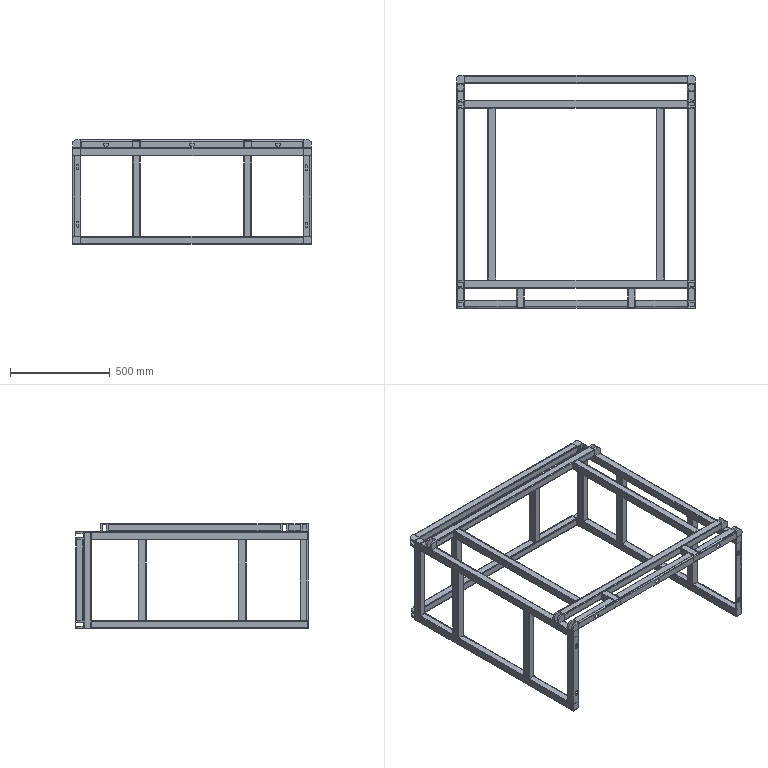Part | SolidWorks | features ReferencePattern 21, MirrorCompFeat 7, LocalLPattern 2 | 48 solids | 627 faces | box 1196 x 1166 x 524.14 mm | volume 5123643 mm3 | plane 404 | cylinder 223 | commonest cylinder face diameters 8 x87 4 x80 14 x29 40 x16 2.667 x4 26 x4